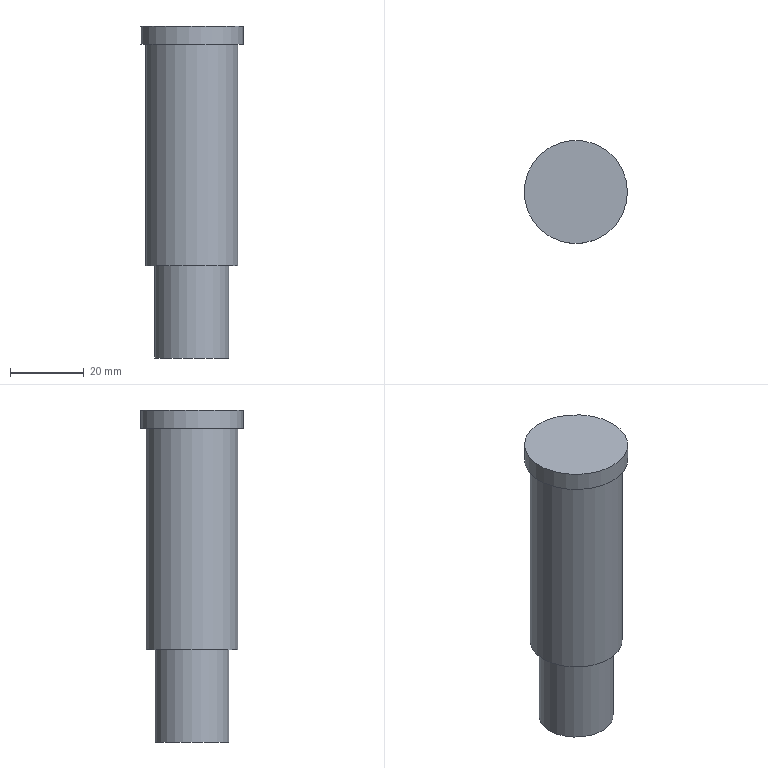Part | NX | features solid 2 | 1 solid | 7 faces | box 28 x 28 x 90 mm | volume 40464 mm3 | plane 4 | cylinder 3 | commonest cylinder face diameters 20.1 x1 25 x1 28 x1
STEP:
#1=CARTESIAN_POINT('',(-618.216,513.153,32.));
#2=VERTEX_POINT('',#1);
#3=CARTESIAN_POINT('',(-630.716,513.153,32.));
#4=DIRECTION('',(0.,0.,-1.));
#5=DIRECTION('',(1.,0.,0.));
#6=AXIS2_PLACEMENT_3D('',#3,#4,#5);
#7=CIRCLE('',#6,12.5);
#8=EDGE_CURVE('',#2,#2,#7,.T.);
#9=ORIENTED_EDGE('',*,*,#8,.F.);
#10=EDGE_LOOP('',(#9));
#11=FACE_BOUND('',#10,.T.);
#12=CARTESIAN_POINT('',(-618.216,513.153,92.));
#13=VERTEX_POINT('',#12);
#14=CARTESIAN_POINT('',(-630.716,513.153,92.));
#15=DIRECTION('',(0.,0.,-1.));
#16=DIRECTION('',(1.,0.,0.));
#17=AXIS2_PLACEMENT_3D('',#14,#15,#16);
#18=CIRCLE('',#17,12.5);
#19=EDGE_CURVE('',#13,#13,#18,.T.);
#20=ORIENTED_EDGE('',*,*,#19,.T.);
#21=EDGE_LOOP('',(#20));
#22=FACE_BOUND('',#21,.T.);
#23=CARTESIAN_POINT('',(-630.716,513.153,97.));
#24=DIRECTION('',(0.,0.,-1.));
#25=DIRECTION('',(-1.,0.,0.));
#26=AXIS2_PLACEMENT_3D('',#23,#24,#25);
#27=CYLINDRICAL_SURFACE('',#26,12.5);
#28=ADVANCED_FACE('',(#11,#22),#27,.T.);
#29=CARTESIAN_POINT('',(-620.666,513.153,32.));
#30=VERTEX_POINT('',#29);
#31=CARTESIAN_POINT('',(-630.716,513.153,32.));
#32=DIRECTION('',(0.,0.,-1.));
#33=DIRECTION('',(1.,0.,0.));
#34=AXIS2_PLACEMENT_3D('',#31,#32,#33);
#35=CIRCLE('',#34,10.05);
#36=EDGE_CURVE('',#30,#30,#35,.T.);
#37=ORIENTED_EDGE('',*,*,#36,.F.);
#38=EDGE_LOOP('',(#37));
#39=FACE_BOUND('',#38,.T.);
#40=ORIENTED_EDGE('',*,*,#8,.T.);
#41=EDGE_LOOP('',(#40));
#42=FACE_BOUND('',#41,.T.);
#43=CARTESIAN_POINT('',(-630.716,513.153,32.));
#44=DIRECTION('',(0.,0.,1.));
#45=DIRECTION('',(1.,0.,0.));
#46=AXIS2_PLACEMENT_3D('',#43,#44,#45);
#47=PLANE('',#46);
#48=ADVANCED_FACE('',(#39,#42),#47,.F.);
#49=CARTESIAN_POINT('',(-616.716,513.153,92.));
#50=VERTEX_POINT('',#49);
#51=CARTESIAN_POINT('',(-630.716,513.153,92.));
#52=DIRECTION('',(0.,0.,-1.));
#53=DIRECTION('',(1.,0.,0.));
#54=AXIS2_PLACEMENT_3D('',#51,#52,#53);
#55=CIRCLE('',#54,14.);
#56=EDGE_CURVE('',#50,#50,#55,.T.);
#57=ORIENTED_EDGE('',*,*,#56,.T.);
#58=EDGE_LOOP('',(#57));
#59=FACE_BOUND('',#58,.T.);
#60=ORIENTED_EDGE('',*,*,#19,.F.);
#61=EDGE_LOOP('',(#60));
#62=FACE_BOUND('',#61,.T.);
#63=CARTESIAN_POINT('',(-630.716,513.153,92.));
#64=DIRECTION('',(0.,0.,1.));
#65=DIRECTION('',(1.,0.,0.));
#66=AXIS2_PLACEMENT_3D('',#63,#64,#65);
#67=PLANE('',#66);
#68=ADVANCED_FACE('',(#59,#62),#67,.F.);
#69=ORIENTED_EDGE('',*,*,#56,.F.);
#70=EDGE_LOOP('',(#69));
#71=FACE_BOUND('',#70,.T.);
#72=CARTESIAN_POINT('',(-616.716,513.153,97.));
#73=VERTEX_POINT('',#72);
#74=CARTESIAN_POINT('',(-630.716,513.153,97.));
#75=DIRECTION('',(0.,0.,-1.));
#76=DIRECTION('',(1.,0.,0.));
#77=AXIS2_PLACEMENT_3D('',#74,#75,#76);
#78=CIRCLE('',#77,14.);
#79=EDGE_CURVE('',#73,#73,#78,.T.);
#80=ORIENTED_EDGE('',*,*,#79,.T.);
#81=EDGE_LOOP('',(#80));
#82=FACE_BOUND('',#81,.T.);
#83=CARTESIAN_POINT('',(-630.716,513.153,92.));
#84=DIRECTION('',(0.,0.,1.));
#85=DIRECTION('',(1.,0.,0.));
#86=AXIS2_PLACEMENT_3D('',#83,#84,#85);
#87=CYLINDRICAL_SURFACE('',#86,14.);
#88=ADVANCED_FACE('',(#71,#82),#87,.T.);
#89=ORIENTED_EDGE('',*,*,#79,.F.);
#90=EDGE_LOOP('',(#89));
#91=FACE_BOUND('',#90,.T.);
#92=CARTESIAN_POINT('',(-630.716,513.153,97.));
#93=DIRECTION('',(0.,0.,1.));
#94=DIRECTION('',(1.,0.,0.));
#95=AXIS2_PLACEMENT_3D('',#92,#93,#94);
#96=PLANE('',#95);
#97=ADVANCED_FACE('',(#91),#96,.T.);
#98=CARTESIAN_POINT('',(-620.666,513.153,7.));
#99=VERTEX_POINT('',#98);
#100=CARTESIAN_POINT('',(-630.716,513.153,7.));
#101=DIRECTION('',(0.,0.,-1.));
#102=DIRECTION('',(1.,0.,0.));
#103=AXIS2_PLACEMENT_3D('',#100,#101,#102);
#104=CIRCLE('',#103,10.05);
#105=EDGE_CURVE('',#99,#99,#104,.T.);
#106=ORIENTED_EDGE('',*,*,#105,.F.);
#107=EDGE_LOOP('',(#106));
#108=FACE_BOUND('',#107,.T.);
#109=ORIENTED_EDGE('',*,*,#36,.T.);
#110=EDGE_LOOP('',(#109));
#111=FACE_BOUND('',#110,.T.);
#112=CARTESIAN_POINT('',(-630.716,513.153,7.));
#113=DIRECTION('',(0.,0.,1.));
#114=DIRECTION('',(1.,0.,0.));
#115=AXIS2_PLACEMENT_3D('',#112,#113,#114);
#116=CYLINDRICAL_SURFACE('',#115,10.05);
#117=ADVANCED_FACE('',(#108,#111),#116,.T.);
#118=ORIENTED_EDGE('',*,*,#105,.T.);
#119=EDGE_LOOP('',(#118));
#120=FACE_BOUND('',#119,.T.);
#121=CARTESIAN_POINT('',(-630.716,513.153,7.));
#122=DIRECTION('',(0.,0.,1.));
#123=DIRECTION('',(1.,0.,0.));
#124=AXIS2_PLACEMENT_3D('',#121,#122,#123);
#125=PLANE('',#124);
#126=ADVANCED_FACE('',(#120),#125,.F.);
#127=CLOSED_SHELL('',(#28,#48,#68,#88,#97,#117,#126));
#128=MANIFOLD_SOLID_BREP('',#127);
#129=(LENGTH_UNIT()NAMED_UNIT(*)SI_UNIT(.MILLI.,.METRE.));
#130=UNCERTAINTY_MEASURE_WITH_UNIT(LENGTH_MEASURE(0.00001),#129,'','');
#131=(NAMED_UNIT(*)PLANE_ANGLE_UNIT()SI_UNIT($,.RADIAN.));
#132=(NAMED_UNIT(*)SI_UNIT($,.STERADIAN.)SOLID_ANGLE_UNIT());
#133=(GEOMETRIC_REPRESENTATION_CONTEXT(3)GLOBAL_UNCERTAINTY_ASSIGNED_CONTEXT((#130))GLOBAL_UNIT_ASSIGNED_CONTEXT((#129,#131,#132))REPRESENTATION_CONTEXT('',''));
#134=ADVANCED_BREP_SHAPE_REPRESENTATION('',(#128),#133);